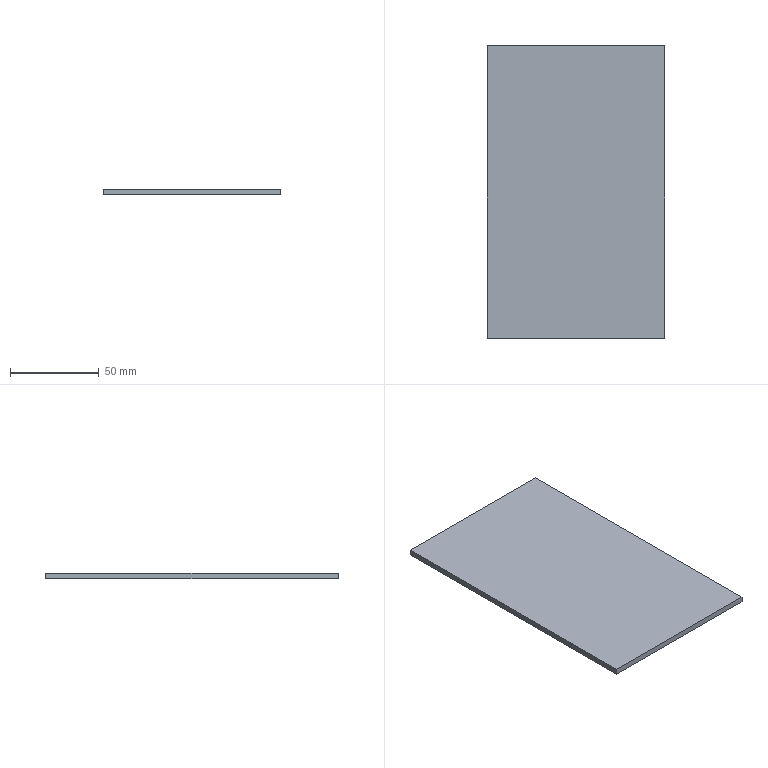Part | STEP file | DMG10600T070_01WTC_X2_8FEA658_5 | 1 solid | 11 faces | box 99.96 x 164.86 x 3.3 mm | volume 52395 mm3 | plane 11
STEP:
#1=CARTESIAN_POINT('',(0.,0.,0.));
#2=DIRECTION('',(0.,0.,1.));
#3=DIRECTION('',(1.,0.,0.));
#4=AXIS2_PLACEMENT_3D('',#1,#2,#3);
#5=CARTESIAN_POINT('',(-49.977,-82.428,-5.7));
#6=VERTEX_POINT('',#5);
#7=CARTESIAN_POINT('',(49.983,-82.428,-5.7));
#8=VERTEX_POINT('',#7);
#9=CARTESIAN_POINT('',(-49.977,-82.428,-5.7));
#10=DIRECTION('',(1.,0.,0.));
#11=VECTOR('',#10,1.);
#12=LINE('',#9,#11);
#13=CARTESIAN_POINT('',(425.814,-2378.632,-5.7));
#14=DIRECTION('',(0.,0.,-1.));
#15=DIRECTION('',(0.,-1.,0.));
#16=AXIS2_PLACEMENT_3D('',#13,#14,#15);
#17=PLANE('',#16);
#18=CARTESIAN_POINT('',(-2296.204,475.791));
#19=DIRECTION('',(0.,-1.));
#20=VECTOR('',#19,1.);
#21=LINE('',#18,#20);
#22=(GEOMETRIC_REPRESENTATION_CONTEXT(2)PARAMETRIC_REPRESENTATION_CONTEXT()REPRESENTATION_CONTEXT('',''));
#23=DEFINITIONAL_REPRESENTATION('',(#21),#22);
#24=PCURVE('',#17,#23);
#25=CARTESIAN_POINT('',(49.983,-82.428,-5.7));
#26=DIRECTION('',(0.,-1.,0.));
#27=DIRECTION('',(1.,0.,0.));
#28=AXIS2_PLACEMENT_3D('',#25,#26,#27);
#29=PLANE('',#28);
#30=CARTESIAN_POINT('',(-99.96,0.));
#31=DIRECTION('',(1.,0.));
#32=VECTOR('',#31,1.);
#33=LINE('',#30,#32);
#34=(GEOMETRIC_REPRESENTATION_CONTEXT(2)PARAMETRIC_REPRESENTATION_CONTEXT()REPRESENTATION_CONTEXT('',''));
#35=DEFINITIONAL_REPRESENTATION('',(#33),#34);
#36=PCURVE('',#29,#35);
#37=SURFACE_CURVE('',#12,(#24,#36),.PCURVE_S1.);
#38=EDGE_CURVE('',#6,#8,#37,.T.);
#39=ORIENTED_EDGE('',*,*,#38,.T.);
#40=CARTESIAN_POINT('',(49.983,82.432,-5.7));
#41=VERTEX_POINT('',#40);
#42=CARTESIAN_POINT('',(49.983,-82.428,-5.7));
#43=DIRECTION('',(0.,1.,0.));
#44=VECTOR('',#43,1.);
#45=LINE('',#42,#44);
#46=CARTESIAN_POINT('',(-2296.204,375.831));
#47=DIRECTION('',(-1.,0.));
#48=VECTOR('',#47,1.);
#49=LINE('',#46,#48);
#50=(GEOMETRIC_REPRESENTATION_CONTEXT(2)PARAMETRIC_REPRESENTATION_CONTEXT()REPRESENTATION_CONTEXT('',''));
#51=DEFINITIONAL_REPRESENTATION('',(#49),#50);
#52=PCURVE('',#17,#51);
#53=CARTESIAN_POINT('',(49.983,82.432,-5.7));
#54=DIRECTION('',(1.,0.,0.));
#55=DIRECTION('',(0.,1.,0.));
#56=AXIS2_PLACEMENT_3D('',#53,#54,#55);
#57=PLANE('',#56);
#58=CARTESIAN_POINT('',(-164.86,0.));
#59=DIRECTION('',(1.,0.));
#60=VECTOR('',#59,1.);
#61=LINE('',#58,#60);
#62=(GEOMETRIC_REPRESENTATION_CONTEXT(2)PARAMETRIC_REPRESENTATION_CONTEXT()REPRESENTATION_CONTEXT('',''));
#63=DEFINITIONAL_REPRESENTATION('',(#61),#62);
#64=PCURVE('',#57,#63);
#65=SURFACE_CURVE('',#45,(#52,#64),.PCURVE_S1.);
#66=EDGE_CURVE('',#8,#41,#65,.T.);
#67=ORIENTED_EDGE('',*,*,#66,.T.);
#68=CARTESIAN_POINT('',(-49.977,82.432,-5.7));
#69=VERTEX_POINT('',#68);
#70=CARTESIAN_POINT('',(49.983,82.432,-5.7));
#71=DIRECTION('',(-1.,0.,0.));
#72=VECTOR('',#71,1.);
#73=LINE('',#70,#72);
#74=CARTESIAN_POINT('',(-2461.064,375.831));
#75=DIRECTION('',(0.,1.));
#76=VECTOR('',#75,1.);
#77=LINE('',#74,#76);
#78=(GEOMETRIC_REPRESENTATION_CONTEXT(2)PARAMETRIC_REPRESENTATION_CONTEXT()REPRESENTATION_CONTEXT('',''));
#79=DEFINITIONAL_REPRESENTATION('',(#77),#78);
#80=PCURVE('',#17,#79);
#81=CARTESIAN_POINT('',(-49.977,82.432,-5.7));
#82=DIRECTION('',(0.,1.,0.));
#83=DIRECTION('',(-1.,0.,0.));
#84=AXIS2_PLACEMENT_3D('',#81,#82,#83);
#85=PLANE('',#84);
#86=CARTESIAN_POINT('',(-99.96,0.));
#87=DIRECTION('',(1.,0.));
#88=VECTOR('',#87,1.);
#89=LINE('',#86,#88);
#90=(GEOMETRIC_REPRESENTATION_CONTEXT(2)PARAMETRIC_REPRESENTATION_CONTEXT()REPRESENTATION_CONTEXT('',''));
#91=DEFINITIONAL_REPRESENTATION('',(#89),#90);
#92=PCURVE('',#85,#91);
#93=SURFACE_CURVE('',#73,(#80,#92),.PCURVE_S1.);
#94=EDGE_CURVE('',#41,#69,#93,.T.);
#95=ORIENTED_EDGE('',*,*,#94,.T.);
#96=CARTESIAN_POINT('',(-49.977,82.432,-5.7));
#97=DIRECTION('',(0.,-1.,0.));
#98=VECTOR('',#97,1.);
#99=LINE('',#96,#98);
#100=CARTESIAN_POINT('',(-2461.064,475.791));
#101=DIRECTION('',(1.,0.));
#102=VECTOR('',#101,1.);
#103=LINE('',#100,#102);
#104=(GEOMETRIC_REPRESENTATION_CONTEXT(2)PARAMETRIC_REPRESENTATION_CONTEXT()REPRESENTATION_CONTEXT('',''));
#105=DEFINITIONAL_REPRESENTATION('',(#103),#104);
#106=PCURVE('',#17,#105);
#107=CARTESIAN_POINT('',(-49.977,-82.428,-5.7));
#108=DIRECTION('',(-1.,0.,0.));
#109=DIRECTION('',(0.,-1.,0.));
#110=AXIS2_PLACEMENT_3D('',#107,#108,#109);
#111=PLANE('',#110);
#112=CARTESIAN_POINT('',(-164.86,0.));
#113=DIRECTION('',(1.,0.));
#114=VECTOR('',#113,1.);
#115=LINE('',#112,#114);
#116=(GEOMETRIC_REPRESENTATION_CONTEXT(2)PARAMETRIC_REPRESENTATION_CONTEXT()REPRESENTATION_CONTEXT('',''));
#117=DEFINITIONAL_REPRESENTATION('',(#115),#116);
#118=PCURVE('',#111,#117);
#119=SURFACE_CURVE('',#99,(#106,#118),.PCURVE_S1.);
#120=EDGE_CURVE('',#69,#6,#119,.T.);
#121=ORIENTED_EDGE('',*,*,#120,.T.);
#122=EDGE_LOOP('',(#39,#67,#95,#121));
#123=FACE_BOUND('',#122,.F.);
#124=CARTESIAN_POINT('',(45.113,-78.905,-5.7));
#125=VERTEX_POINT('',#124);
#126=CARTESIAN_POINT('',(45.113,75.309,-5.7));
#127=VERTEX_POINT('',#126);
#128=CARTESIAN_POINT('',(45.113,-78.905,-5.7));
#129=DIRECTION('',(0.,1.,0.));
#130=VECTOR('',#129,1.);
#131=LINE('',#128,#130);
#132=CARTESIAN_POINT('',(-2299.727,380.701));
#133=DIRECTION('',(-1.,0.));
#134=VECTOR('',#133,1.);
#135=LINE('',#132,#134);
#136=(GEOMETRIC_REPRESENTATION_CONTEXT(2)PARAMETRIC_REPRESENTATION_CONTEXT()REPRESENTATION_CONTEXT('',''));
#137=DEFINITIONAL_REPRESENTATION('',(#135),#136);
#138=PCURVE('',#17,#137);
#139=CARTESIAN_POINT('',(45.113,75.309,-5.7));
#140=DIRECTION('',(1.,0.,0.));
#141=DIRECTION('',(0.,1.,0.));
#142=AXIS2_PLACEMENT_3D('',#139,#140,#141);
#143=PLANE('',#142);
#144=CARTESIAN_POINT('',(-154.214,0.));
#145=DIRECTION('',(1.,0.));
#146=VECTOR('',#145,1.);
#147=LINE('',#144,#146);
#148=(GEOMETRIC_REPRESENTATION_CONTEXT(2)PARAMETRIC_REPRESENTATION_CONTEXT()REPRESENTATION_CONTEXT('',''));
#149=DEFINITIONAL_REPRESENTATION('',(#147),#148);
#150=PCURVE('',#143,#149);
#151=SURFACE_CURVE('',#131,(#138,#150),.PCURVE_S1.);
#152=EDGE_CURVE('',#125,#127,#151,.T.);
#153=ORIENTED_EDGE('',*,*,#152,.F.);
#154=CARTESIAN_POINT('',(-40.807,-78.905,-5.7));
#155=VERTEX_POINT('',#154);
#156=CARTESIAN_POINT('',(-40.807,-78.905,-5.7));
#157=DIRECTION('',(1.,0.,0.));
#158=VECTOR('',#157,1.);
#159=LINE('',#156,#158);
#160=CARTESIAN_POINT('',(-2299.727,466.621));
#161=DIRECTION('',(0.,-1.));
#162=VECTOR('',#161,1.);
#163=LINE('',#160,#162);
#164=(GEOMETRIC_REPRESENTATION_CONTEXT(2)PARAMETRIC_REPRESENTATION_CONTEXT()REPRESENTATION_CONTEXT('',''));
#165=DEFINITIONAL_REPRESENTATION('',(#163),#164);
#166=PCURVE('',#17,#165);
#167=CARTESIAN_POINT('',(45.113,-78.905,-5.7));
#168=DIRECTION('',(0.,-1.,0.));
#169=DIRECTION('',(1.,0.,0.));
#170=AXIS2_PLACEMENT_3D('',#167,#168,#169);
#171=PLANE('',#170);
#172=CARTESIAN_POINT('',(-85.92,0.));
#173=DIRECTION('',(1.,0.));
#174=VECTOR('',#173,1.);
#175=LINE('',#172,#174);
#176=(GEOMETRIC_REPRESENTATION_CONTEXT(2)PARAMETRIC_REPRESENTATION_CONTEXT()REPRESENTATION_CONTEXT('',''));
#177=DEFINITIONAL_REPRESENTATION('',(#175),#176);
#178=PCURVE('',#171,#177);
#179=SURFACE_CURVE('',#159,(#166,#178),.PCURVE_S1.);
#180=EDGE_CURVE('',#155,#125,#179,.T.);
#181=ORIENTED_EDGE('',*,*,#180,.F.);
#182=CARTESIAN_POINT('',(-40.807,75.309,-5.7));
#183=VERTEX_POINT('',#182);
#184=CARTESIAN_POINT('',(-40.807,75.309,-5.7));
#185=DIRECTION('',(0.,-1.,0.));
#186=VECTOR('',#185,1.);
#187=LINE('',#184,#186);
#188=CARTESIAN_POINT('',(-2453.941,466.621));
#189=DIRECTION('',(1.,0.));
#190=VECTOR('',#189,1.);
#191=LINE('',#188,#190);
#192=(GEOMETRIC_REPRESENTATION_CONTEXT(2)PARAMETRIC_REPRESENTATION_CONTEXT()REPRESENTATION_CONTEXT('',''));
#193=DEFINITIONAL_REPRESENTATION('',(#191),#192);
#194=PCURVE('',#17,#193);
#195=CARTESIAN_POINT('',(-40.807,-78.905,-5.7));
#196=DIRECTION('',(-1.,0.,0.));
#197=DIRECTION('',(0.,-1.,0.));
#198=AXIS2_PLACEMENT_3D('',#195,#196,#197);
#199=PLANE('',#198);
#200=CARTESIAN_POINT('',(-154.214,0.));
#201=DIRECTION('',(1.,0.));
#202=VECTOR('',#201,1.);
#203=LINE('',#200,#202);
#204=(GEOMETRIC_REPRESENTATION_CONTEXT(2)PARAMETRIC_REPRESENTATION_CONTEXT()REPRESENTATION_CONTEXT('',''));
#205=DEFINITIONAL_REPRESENTATION('',(#203),#204);
#206=PCURVE('',#199,#205);
#207=SURFACE_CURVE('',#187,(#194,#206),.PCURVE_S1.);
#208=EDGE_CURVE('',#183,#155,#207,.T.);
#209=ORIENTED_EDGE('',*,*,#208,.F.);
#210=CARTESIAN_POINT('',(45.113,75.309,-5.7));
#211=DIRECTION('',(-1.,0.,0.));
#212=VECTOR('',#211,1.);
#213=LINE('',#210,#212);
#214=CARTESIAN_POINT('',(-2453.941,380.701));
#215=DIRECTION('',(0.,1.));
#216=VECTOR('',#215,1.);
#217=LINE('',#214,#216);
#218=(GEOMETRIC_REPRESENTATION_CONTEXT(2)PARAMETRIC_REPRESENTATION_CONTEXT()REPRESENTATION_CONTEXT('',''));
#219=DEFINITIONAL_REPRESENTATION('',(#217),#218);
#220=PCURVE('',#17,#219);
#221=CARTESIAN_POINT('',(-40.807,75.309,-5.7));
#222=DIRECTION('',(0.,1.,0.));
#223=DIRECTION('',(-1.,0.,0.));
#224=AXIS2_PLACEMENT_3D('',#221,#222,#223);
#225=PLANE('',#224);
#226=CARTESIAN_POINT('',(-85.92,0.));
#227=DIRECTION('',(1.,0.));
#228=VECTOR('',#227,1.);
#229=LINE('',#226,#228);
#230=(GEOMETRIC_REPRESENTATION_CONTEXT(2)PARAMETRIC_REPRESENTATION_CONTEXT()REPRESENTATION_CONTEXT('',''));
#231=DEFINITIONAL_REPRESENTATION('',(#229),#230);
#232=PCURVE('',#225,#231);
#233=SURFACE_CURVE('',#213,(#220,#232),.PCURVE_S1.);
#234=EDGE_CURVE('',#127,#183,#233,.T.);
#235=ORIENTED_EDGE('',*,*,#234,.F.);
#236=EDGE_LOOP('',(#153,#181,#209,#235));
#237=FACE_BOUND('',#236,.F.);
#238=ADVANCED_FACE('',(#123,#237),#17,.T.);
#239=CARTESIAN_POINT('',(49.983,-82.428,-2.4));
#240=VERTEX_POINT('',#239);
#241=CARTESIAN_POINT('',(49.983,-82.428,-2.4));
#242=DIRECTION('',(0.,0.,-1.));
#243=VECTOR('',#242,1.);
#244=LINE('',#241,#243);
#245=CARTESIAN_POINT('',(0.,3.3));
#246=DIRECTION('',(0.,-1.));
#247=VECTOR('',#246,1.);
#248=LINE('',#245,#247);
#249=(GEOMETRIC_REPRESENTATION_CONTEXT(2)PARAMETRIC_REPRESENTATION_CONTEXT()REPRESENTATION_CONTEXT('',''));
#250=DEFINITIONAL_REPRESENTATION('',(#248),#249);
#251=PCURVE('',#29,#250);
#252=CARTESIAN_POINT('',(-164.86,3.3));
#253=DIRECTION('',(0.,-1.));
#254=VECTOR('',#253,1.);
#255=LINE('',#252,#254);
#256=(GEOMETRIC_REPRESENTATION_CONTEXT(2)PARAMETRIC_REPRESENTATION_CONTEXT()REPRESENTATION_CONTEXT('',''));
#257=DEFINITIONAL_REPRESENTATION('',(#255),#256);
#258=PCURVE('',#57,#257);
#259=SURFACE_CURVE('',#244,(#251,#258),.PCURVE_S1.);
#260=EDGE_CURVE('',#240,#8,#259,.T.);
#261=ORIENTED_EDGE('',*,*,#260,.T.);
#262=ORIENTED_EDGE('',*,*,#38,.F.);
#263=CARTESIAN_POINT('',(-49.977,-82.428,-2.4));
#264=VERTEX_POINT('',#263);
#265=CARTESIAN_POINT('',(-49.977,-82.428,-2.4));
#266=DIRECTION('',(0.,0.,-1.));
#267=VECTOR('',#266,1.);
#268=LINE('',#265,#267);
#269=CARTESIAN_POINT('',(-99.96,3.3));
#270=DIRECTION('',(0.,-1.));
#271=VECTOR('',#270,1.);
#272=LINE('',#269,#271);
#273=(GEOMETRIC_REPRESENTATION_CONTEXT(2)PARAMETRIC_REPRESENTATION_CONTEXT()REPRESENTATION_CONTEXT('',''));
#274=DEFINITIONAL_REPRESENTATION('',(#272),#273);
#275=PCURVE('',#29,#274);
#276=CARTESIAN_POINT('',(0.,3.3));
#277=DIRECTION('',(0.,-1.));
#278=VECTOR('',#277,1.);
#279=LINE('',#276,#278);
#280=(GEOMETRIC_REPRESENTATION_CONTEXT(2)PARAMETRIC_REPRESENTATION_CONTEXT()REPRESENTATION_CONTEXT('',''));
#281=DEFINITIONAL_REPRESENTATION('',(#279),#280);
#282=PCURVE('',#111,#281);
#283=SURFACE_CURVE('',#268,(#275,#282),.PCURVE_S1.);
#284=EDGE_CURVE('',#264,#6,#283,.T.);
#285=ORIENTED_EDGE('',*,*,#284,.F.);
#286=CARTESIAN_POINT('',(-49.977,-82.428,-2.4));
#287=DIRECTION('',(1.,0.,0.));
#288=VECTOR('',#287,1.);
#289=LINE('',#286,#288);
#290=CARTESIAN_POINT('',(-99.96,3.3));
#291=DIRECTION('',(1.,0.));
#292=VECTOR('',#291,1.);
#293=LINE('',#290,#292);
#294=(GEOMETRIC_REPRESENTATION_CONTEXT(2)PARAMETRIC_REPRESENTATION_CONTEXT()REPRESENTATION_CONTEXT('',''));
#295=DEFINITIONAL_REPRESENTATION('',(#293),#294);
#296=PCURVE('',#29,#295);
#297=CARTESIAN_POINT('',(425.814,-2378.632,-2.4));
#298=DIRECTION('',(0.,0.,-1.));
#299=DIRECTION('',(0.,-1.,0.));
#300=AXIS2_PLACEMENT_3D('',#297,#298,#299);
#301=PLANE('',#300);
#302=CARTESIAN_POINT('',(-2296.204,475.791));
#303=DIRECTION('',(0.,-1.));
#304=VECTOR('',#303,1.);
#305=LINE('',#302,#304);
#306=(GEOMETRIC_REPRESENTATION_CONTEXT(2)PARAMETRIC_REPRESENTATION_CONTEXT()REPRESENTATION_CONTEXT('',''));
#307=DEFINITIONAL_REPRESENTATION('',(#305),#306);
#308=PCURVE('',#301,#307);
#309=SURFACE_CURVE('',#289,(#296,#308),.PCURVE_S1.);
#310=EDGE_CURVE('',#264,#240,#309,.T.);
#311=ORIENTED_EDGE('',*,*,#310,.T.);
#312=EDGE_LOOP('',(#261,#262,#285,#311));
#313=FACE_BOUND('',#312,.F.);
#314=ADVANCED_FACE('',(#313),#29,.T.);
#315=CARTESIAN_POINT('',(49.983,82.432,-2.4));
#316=VERTEX_POINT('',#315);
#317=CARTESIAN_POINT('',(49.983,82.432,-2.4));
#318=DIRECTION('',(0.,0.,-1.));
#319=VECTOR('',#318,1.);
#320=LINE('',#317,#319);
#321=CARTESIAN_POINT('',(0.,3.3));
#322=DIRECTION('',(0.,-1.));
#323=VECTOR('',#322,1.);
#324=LINE('',#321,#323);
#325=(GEOMETRIC_REPRESENTATION_CONTEXT(2)PARAMETRIC_REPRESENTATION_CONTEXT()REPRESENTATION_CONTEXT('',''));
#326=DEFINITIONAL_REPRESENTATION('',(#324),#325);
#327=PCURVE('',#57,#326);
#328=CARTESIAN_POINT('',(-99.96,3.3));
#329=DIRECTION('',(0.,-1.));
#330=VECTOR('',#329,1.);
#331=LINE('',#328,#330);
#332=(GEOMETRIC_REPRESENTATION_CONTEXT(2)PARAMETRIC_REPRESENTATION_CONTEXT()REPRESENTATION_CONTEXT('',''));
#333=DEFINITIONAL_REPRESENTATION('',(#331),#332);
#334=PCURVE('',#85,#333);
#335=SURFACE_CURVE('',#320,(#327,#334),.PCURVE_S1.);
#336=EDGE_CURVE('',#316,#41,#335,.T.);
#337=ORIENTED_EDGE('',*,*,#336,.T.);
#338=ORIENTED_EDGE('',*,*,#66,.F.);
#339=ORIENTED_EDGE('',*,*,#260,.F.);
#340=CARTESIAN_POINT('',(49.983,-82.428,-2.4));
#341=DIRECTION('',(0.,1.,0.));
#342=VECTOR('',#341,1.);
#343=LINE('',#340,#342);
#344=CARTESIAN_POINT('',(-164.86,3.3));
#345=DIRECTION('',(1.,0.));
#346=VECTOR('',#345,1.);
#347=LINE('',#344,#346);
#348=(GEOMETRIC_REPRESENTATION_CONTEXT(2)PARAMETRIC_REPRESENTATION_CONTEXT()REPRESENTATION_CONTEXT('',''));
#349=DEFINITIONAL_REPRESENTATION('',(#347),#348);
#350=PCURVE('',#57,#349);
#351=CARTESIAN_POINT('',(-2296.204,375.831));
#352=DIRECTION('',(-1.,0.));
#353=VECTOR('',#352,1.);
#354=LINE('',#351,#353);
#355=(GEOMETRIC_REPRESENTATION_CONTEXT(2)PARAMETRIC_REPRESENTATION_CONTEXT()REPRESENTATION_CONTEXT('',''));
#356=DEFINITIONAL_REPRESENTATION('',(#354),#355);
#357=PCURVE('',#301,#356);
#358=SURFACE_CURVE('',#343,(#350,#357),.PCURVE_S1.);
#359=EDGE_CURVE('',#240,#316,#358,.T.);
#360=ORIENTED_EDGE('',*,*,#359,.T.);
#361=EDGE_LOOP('',(#337,#338,#339,#360));
#362=FACE_BOUND('',#361,.F.);
#363=ADVANCED_FACE('',(#362),#57,.T.);
#364=CARTESIAN_POINT('',(-49.977,82.432,-2.4));
#365=VERTEX_POINT('',#364);
#366=CARTESIAN_POINT('',(-49.977,82.432,-2.4));
#367=DIRECTION('',(0.,0.,-1.));
#368=VECTOR('',#367,1.);
#369=LINE('',#366,#368);
#370=CARTESIAN_POINT('',(0.,3.3));
#371=DIRECTION('',(0.,-1.));
#372=VECTOR('',#371,1.);
#373=LINE('',#370,#372);
#374=(GEOMETRIC_REPRESENTATION_CONTEXT(2)PARAMETRIC_REPRESENTATION_CONTEXT()REPRESENTATION_CONTEXT('',''));
#375=DEFINITIONAL_REPRESENTATION('',(#373),#374);
#376=PCURVE('',#85,#375);
#377=CARTESIAN_POINT('',(-164.86,3.3));
#378=DIRECTION('',(0.,-1.));
#379=VECTOR('',#378,1.);
#380=LINE('',#377,#379);
#381=(GEOMETRIC_REPRESENTATION_CONTEXT(2)PARAMETRIC_REPRESENTATION_CONTEXT()REPRESENTATION_CONTEXT('',''));
#382=DEFINITIONAL_REPRESENTATION('',(#380),#381);
#383=PCURVE('',#111,#382);
#384=SURFACE_CURVE('',#369,(#376,#383),.PCURVE_S1.);
#385=EDGE_CURVE('',#365,#69,#384,.T.);
#386=ORIENTED_EDGE('',*,*,#385,.T.);
#387=ORIENTED_EDGE('',*,*,#94,.F.);
#388=ORIENTED_EDGE('',*,*,#336,.F.);
#389=CARTESIAN_POINT('',(49.983,82.432,-2.4));
#390=DIRECTION('',(-1.,0.,0.));
#391=VECTOR('',#390,1.);
#392=LINE('',#389,#391);
#393=CARTESIAN_POINT('',(-99.96,3.3));
#394=DIRECTION('',(1.,0.));
#395=VECTOR('',#394,1.);
#396=LINE('',#393,#395);
#397=(GEOMETRIC_REPRESENTATION_CONTEXT(2)PARAMETRIC_REPRESENTATION_CONTEXT()REPRESENTATION_CONTEXT('',''));
#398=DEFINITIONAL_REPRESENTATION('',(#396),#397);
#399=PCURVE('',#85,#398);
#400=CARTESIAN_POINT('',(-2461.064,375.831));
#401=DIRECTION('',(0.,1.));
#402=VECTOR('',#401,1.);
#403=LINE('',#400,#402);
#404=(GEOMETRIC_REPRESENTATION_CONTEXT(2)PARAMETRIC_REPRESENTATION_CONTEXT()REPRESENTATION_CONTEXT('',''));
#405=DEFINITIONAL_REPRESENTATION('',(#403),#404);
#406=PCURVE('',#301,#405);
#407=SURFACE_CURVE('',#392,(#399,#406),.PCURVE_S1.);
#408=EDGE_CURVE('',#316,#365,#407,.T.);
#409=ORIENTED_EDGE('',*,*,#408,.T.);
#410=EDGE_LOOP('',(#386,#387,#388,#409));
#411=FACE_BOUND('',#410,.F.);
#412=ADVANCED_FACE('',(#411),#85,.T.);
#413=ORIENTED_EDGE('',*,*,#284,.T.);
#414=ORIENTED_EDGE('',*,*,#120,.F.);
#415=ORIENTED_EDGE('',*,*,#385,.F.);
#416=CARTESIAN_POINT('',(-49.977,82.432,-2.4));
#417=DIRECTION('',(0.,-1.,0.));
#418=VECTOR('',#417,1.);
#419=LINE('',#416,#418);
#420=CARTESIAN_POINT('',(-164.86,3.3));
#421=DIRECTION('',(1.,0.));
#422=VECTOR('',#421,1.);
#423=LINE('',#420,#422);
#424=(GEOMETRIC_REPRESENTATION_CONTEXT(2)PARAMETRIC_REPRESENTATION_CONTEXT()REPRESENTATION_CONTEXT('',''));
#425=DEFINITIONAL_REPRESENTATION('',(#423),#424);
#426=PCURVE('',#111,#425);
#427=CARTESIAN_POINT('',(-2461.064,475.791));
#428=DIRECTION('',(1.,0.));
#429=VECTOR('',#428,1.);
#430=LINE('',#427,#429);
#431=(GEOMETRIC_REPRESENTATION_CONTEXT(2)PARAMETRIC_REPRESENTATION_CONTEXT()REPRESENTATION_CONTEXT('',''));
#432=DEFINITIONAL_REPRESENTATION('',(#430),#431);
#433=PCURVE('',#301,#432);
#434=SURFACE_CURVE('',#419,(#426,#433),.PCURVE_S1.);
#435=EDGE_CURVE('',#365,#264,#434,.T.);
#436=ORIENTED_EDGE('',*,*,#435,.T.);
#437=EDGE_LOOP('',(#413,#414,#415,#436));
#438=FACE_BOUND('',#437,.F.);
#439=ADVANCED_FACE('',(#438),#111,.T.);
#440=ORIENTED_EDGE('',*,*,#408,.F.);
#441=ORIENTED_EDGE('',*,*,#359,.F.);
#442=ORIENTED_EDGE('',*,*,#310,.F.);
#443=ORIENTED_EDGE('',*,*,#435,.F.);
#444=EDGE_LOOP('',(#440,#441,#442,#443));
#445=FACE_BOUND('',#444,.F.);
#446=ADVANCED_FACE('',(#445),#301,.F.);
#447=CARTESIAN_POINT('',(45.113,-78.905,-5.55));
#448=VERTEX_POINT('',#447);
#449=CARTESIAN_POINT('',(45.113,-78.905,-5.55));
#450=DIRECTION('',(0.,0.,-1.));
#451=VECTOR('',#450,1.);
#452=LINE('',#449,#451);
#453=CARTESIAN_POINT('',(-154.214,0.15));
#454=DIRECTION('',(0.,-1.));
#455=VECTOR('',#454,1.);
#456=LINE('',#453,#455);
#457=(GEOMETRIC_REPRESENTATION_CONTEXT(2)PARAMETRIC_REPRESENTATION_CONTEXT()REPRESENTATION_CONTEXT('',''));
#458=DEFINITIONAL_REPRESENTATION('',(#456),#457);
#459=PCURVE('',#143,#458);
#460=CARTESIAN_POINT('',(0.,0.15));
#461=DIRECTION('',(0.,-1.));
#462=VECTOR('',#461,1.);
#463=LINE('',#460,#462);
#464=(GEOMETRIC_REPRESENTATION_CONTEXT(2)PARAMETRIC_REPRESENTATION_CONTEXT()REPRESENTATION_CONTEXT('',''));
#465=DEFINITIONAL_REPRESENTATION('',(#463),#464);
#466=PCURVE('',#171,#465);
#467=SURFACE_CURVE('',#452,(#459,#466),.PCURVE_S1.);
#468=EDGE_CURVE('',#448,#125,#467,.T.);
#469=ORIENTED_EDGE('',*,*,#468,.T.);
#470=ORIENTED_EDGE('',*,*,#152,.T.);
#471=CARTESIAN_POINT('',(45.113,75.309,-5.55));
#472=VERTEX_POINT('',#471);
#473=CARTESIAN_POINT('',(45.113,75.309,-5.55));
#474=DIRECTION('',(0.,0.,-1.));
#475=VECTOR('',#474,1.);
#476=LINE('',#473,#475);
#477=CARTESIAN_POINT('',(0.,0.15));
#478=DIRECTION('',(0.,-1.));
#479=VECTOR('',#478,1.);
#480=LINE('',#477,#479);
#481=(GEOMETRIC_REPRESENTATION_CONTEXT(2)PARAMETRIC_REPRESENTATION_CONTEXT()REPRESENTATION_CONTEXT('',''));
#482=DEFINITIONAL_REPRESENTATION('',(#480),#481);
#483=PCURVE('',#143,#482);
#484=CARTESIAN_POINT('',(-85.92,0.15));
#485=DIRECTION('',(0.,-1.));
#486=VECTOR('',#485,1.);
#487=LINE('',#484,#486);
#488=(GEOMETRIC_REPRESENTATION_CONTEXT(2)PARAMETRIC_REPRESENTATION_CONTEXT()REPRESENTATION_CONTEXT('',''));
#489=DEFINITIONAL_REPRESENTATION('',(#487),#488);
#490=PCURVE('',#225,#489);
#491=SURFACE_CURVE('',#476,(#483,#490),.PCURVE_S1.);
#492=EDGE_CURVE('',#472,#127,#491,.T.);
#493=ORIENTED_EDGE('',*,*,#492,.F.);
#494=CARTESIAN_POINT('',(45.113,-78.905,-5.55));
#495=DIRECTION('',(0.,1.,0.));
#496=VECTOR('',#495,1.);
#497=LINE('',#494,#496);
#498=CARTESIAN_POINT('',(-154.214,0.15));
#499=DIRECTION('',(1.,0.));
#500=VECTOR('',#499,1.);
#501=LINE('',#498,#500);
#502=(GEOMETRIC_REPRESENTATION_CONTEXT(2)PARAMETRIC_REPRESENTATION_CONTEXT()REPRESENTATION_CONTEXT('',''));
#503=DEFINITIONAL_REPRESENTATION('',(#501),#502);
#504=PCURVE('',#143,#503);
#505=CARTESIAN_POINT('',(-49.977,-82.428,-5.55));
#506=DIRECTION('',(0.,0.,-1.));
#507=DIRECTION('',(0.,-1.,0.));
#508=AXIS2_PLACEMENT_3D('',#505,#506,#507);
#509=PLANE('',#508);
#510=CARTESIAN_POINT('',(-3.523,-95.09));
#511=DIRECTION('',(-1.,0.));
#512=VECTOR('',#511,1.);
#513=LINE('',#510,#512);
#514=(GEOMETRIC_REPRESENTATION_CONTEXT(2)PARAMETRIC_REPRESENTATION_CONTEXT()REPRESENTATION_CONTEXT('',''));
#515=DEFINITIONAL_REPRESENTATION('',(#513),#514);
#516=PCURVE('',#509,#515);
#517=SURFACE_CURVE('',#497,(#504,#516),.PCURVE_S1.);
#518=EDGE_CURVE('',#448,#472,#517,.T.);
#519=ORIENTED_EDGE('',*,*,#518,.F.);
#520=EDGE_LOOP('',(#469,#470,#493,#519));
#521=FACE_BOUND('',#520,.F.);
#522=ADVANCED_FACE('',(#521),#143,.F.);
#523=CARTESIAN_POINT('',(-40.807,-78.905,-5.55));
#524=VERTEX_POINT('',#523);
#525=CARTESIAN_POINT('',(-40.807,-78.905,-5.55));
#526=DIRECTION('',(0.,0.,-1.));
#527=VECTOR('',#526,1.);
#528=LINE('',#525,#527);
#529=CARTESIAN_POINT('',(-85.92,0.15));
#530=DIRECTION('',(0.,-1.));
#531=VECTOR('',#530,1.);
#532=LINE('',#529,#531);
#533=(GEOMETRIC_REPRESENTATION_CONTEXT(2)PARAMETRIC_REPRESENTATION_CONTEXT()REPRESENTATION_CONTEXT('',''));
#534=DEFINITIONAL_REPRESENTATION('',(#532),#533);
#535=PCURVE('',#171,#534);
#536=CARTESIAN_POINT('',(0.,0.15));
#537=DIRECTION('',(0.,-1.));
#538=VECTOR('',#537,1.);
#539=LINE('',#536,#538);
#540=(GEOMETRIC_REPRESENTATION_CONTEXT(2)PARAMETRIC_REPRESENTATION_CONTEXT()REPRESENTATION_CONTEXT('',''));
#541=DEFINITIONAL_REPRESENTATION('',(#539),#540);
#542=PCURVE('',#199,#541);
#543=SURFACE_CURVE('',#528,(#535,#542),.PCURVE_S1.);
#544=EDGE_CURVE('',#524,#155,#543,.T.);
#545=ORIENTED_EDGE('',*,*,#544,.T.);
#546=ORIENTED_EDGE('',*,*,#180,.T.);
#547=ORIENTED_EDGE('',*,*,#468,.F.);
#548=CARTESIAN_POINT('',(-40.807,-78.905,-5.55));
#549=DIRECTION('',(1.,0.,0.));
#550=VECTOR('',#549,1.);
#551=LINE('',#548,#550);
#552=CARTESIAN_POINT('',(-85.92,0.15));
#553=DIRECTION('',(1.,0.));
#554=VECTOR('',#553,1.);
#555=LINE('',#552,#554);
#556=(GEOMETRIC_REPRESENTATION_CONTEXT(2)PARAMETRIC_REPRESENTATION_CONTEXT()REPRESENTATION_CONTEXT('',''));
#557=DEFINITIONAL_REPRESENTATION('',(#555),#556);
#558=PCURVE('',#171,#557);
#559=CARTESIAN_POINT('',(-3.523,-9.17));
#560=DIRECTION('',(0.,-1.));
#561=VECTOR('',#560,1.);
#562=LINE('',#559,#561);
#563=(GEOMETRIC_REPRESENTATION_CONTEXT(2)PARAMETRIC_REPRESENTATION_CONTEXT()REPRESENTATION_CONTEXT('',''));
#564=DEFINITIONAL_REPRESENTATION('',(#562),#563);
#565=PCURVE('',#509,#564);
#566=SURFACE_CURVE('',#551,(#558,#565),.PCURVE_S1.);
#567=EDGE_CURVE('',#524,#448,#566,.T.);
#568=ORIENTED_EDGE('',*,*,#567,.F.);
#569=EDGE_LOOP('',(#545,#546,#547,#568));
#570=FACE_BOUND('',#569,.F.);
#571=ADVANCED_FACE('',(#570),#171,.F.);
#572=CARTESIAN_POINT('',(-40.807,75.309,-5.55));
#573=VERTEX_POINT('',#572);
#574=CARTESIAN_POINT('',(-40.807,75.309,-5.55));
#575=DIRECTION('',(0.,0.,-1.));
#576=VECTOR('',#575,1.);
#577=LINE('',#574,#576);
#578=CARTESIAN_POINT('',(-154.214,0.15));
#579=DIRECTION('',(0.,-1.));
#580=VECTOR('',#579,1.);
#581=LINE('',#578,#580);
#582=(GEOMETRIC_REPRESENTATION_CONTEXT(2)PARAMETRIC_REPRESENTATION_CONTEXT()REPRESENTATION_CONTEXT('',''));
#583=DEFINITIONAL_REPRESENTATION('',(#581),#582);
#584=PCURVE('',#199,#583);
#585=CARTESIAN_POINT('',(0.,0.15));
#586=DIRECTION('',(0.,-1.));
#587=VECTOR('',#586,1.);
#588=LINE('',#585,#587);
#589=(GEOMETRIC_REPRESENTATION_CONTEXT(2)PARAMETRIC_REPRESENTATION_CONTEXT()REPRESENTATION_CONTEXT('',''));
#590=DEFINITIONAL_REPRESENTATION('',(#588),#589);
#591=PCURVE('',#225,#590);
#592=SURFACE_CURVE('',#577,(#584,#591),.PCURVE_S1.);
#593=EDGE_CURVE('',#573,#183,#592,.T.);
#594=ORIENTED_EDGE('',*,*,#593,.T.);
#595=ORIENTED_EDGE('',*,*,#208,.T.);
#596=ORIENTED_EDGE('',*,*,#544,.F.);
#597=CARTESIAN_POINT('',(-40.807,75.309,-5.55));
#598=DIRECTION('',(0.,-1.,0.));
#599=VECTOR('',#598,1.);
#600=LINE('',#597,#599);
#601=CARTESIAN_POINT('',(-154.214,0.15));
#602=DIRECTION('',(1.,0.));
#603=VECTOR('',#602,1.);
#604=LINE('',#601,#603);
#605=(GEOMETRIC_REPRESENTATION_CONTEXT(2)PARAMETRIC_REPRESENTATION_CONTEXT()REPRESENTATION_CONTEXT('',''));
#606=DEFINITIONAL_REPRESENTATION('',(#604),#605);
#607=PCURVE('',#199,#606);
#608=CARTESIAN_POINT('',(-157.737,-9.17));
#609=DIRECTION('',(1.,0.));
#610=VECTOR('',#609,1.);
#611=LINE('',#608,#610);
#612=(GEOMETRIC_REPRESENTATION_CONTEXT(2)PARAMETRIC_REPRESENTATION_CONTEXT()REPRESENTATION_CONTEXT('',''));
#613=DEFINITIONAL_REPRESENTATION('',(#611),#612);
#614=PCURVE('',#509,#613);
#615=SURFACE_CURVE('',#600,(#607,#614),.PCURVE_S1.);
#616=EDGE_CURVE('',#573,#524,#615,.T.);
#617=ORIENTED_EDGE('',*,*,#616,.F.);
#618=EDGE_LOOP('',(#594,#595,#596,#617));
#619=FACE_BOUND('',#618,.F.);
#620=ADVANCED_FACE('',(#619),#199,.F.);
#621=ORIENTED_EDGE('',*,*,#492,.T.);
#622=ORIENTED_EDGE('',*,*,#234,.T.);
#623=ORIENTED_EDGE('',*,*,#593,.F.);
#624=CARTESIAN_POINT('',(45.113,75.309,-5.55));
#625=DIRECTION('',(-1.,0.,0.));
#626=VECTOR('',#625,1.);
#627=LINE('',#624,#626);
#628=CARTESIAN_POINT('',(-85.92,0.15));
#629=DIRECTION('',(1.,0.));
#630=VECTOR('',#629,1.);
#631=LINE('',#628,#630);
#632=(GEOMETRIC_REPRESENTATION_CONTEXT(2)PARAMETRIC_REPRESENTATION_CONTEXT()REPRESENTATION_CONTEXT('',''));
#633=DEFINITIONAL_REPRESENTATION('',(#631),#632);
#634=PCURVE('',#225,#633);
#635=CARTESIAN_POINT('',(-157.737,-95.09));
#636=DIRECTION('',(0.,1.));
#637=VECTOR('',#636,1.);
#638=LINE('',#635,#637);
#639=(GEOMETRIC_REPRESENTATION_CONTEXT(2)PARAMETRIC_REPRESENTATION_CONTEXT()REPRESENTATION_CONTEXT('',''));
#640=DEFINITIONAL_REPRESENTATION('',(#638),#639);
#641=PCURVE('',#509,#640);
#642=SURFACE_CURVE('',#627,(#634,#641),.PCURVE_S1.);
#643=EDGE_CURVE('',#472,#573,#642,.T.);
#644=ORIENTED_EDGE('',*,*,#643,.F.);
#645=EDGE_LOOP('',(#621,#622,#623,#644));
#646=FACE_BOUND('',#645,.F.);
#647=ADVANCED_FACE('',(#646),#225,.F.);
#648=ORIENTED_EDGE('',*,*,#616,.T.);
#649=ORIENTED_EDGE('',*,*,#567,.T.);
#650=ORIENTED_EDGE('',*,*,#518,.T.);
#651=ORIENTED_EDGE('',*,*,#643,.T.);
#652=EDGE_LOOP('',(#648,#649,#650,#651));
#653=FACE_BOUND('',#652,.F.);
#654=ADVANCED_FACE('',(#653),#509,.T.);
#655=CLOSED_SHELL('',(#238,#314,#363,#412,#439,#446,#522,#571,#620,#647,#654));
#656=MANIFOLD_SOLID_BREP('',#655);
#657=(LENGTH_UNIT()NAMED_UNIT(*)SI_UNIT(.MILLI.,.METRE.));
#658=UNCERTAINTY_MEASURE_WITH_UNIT(LENGTH_MEASURE(0.0000001),#657,'','');
#659=(NAMED_UNIT(*)PLANE_ANGLE_UNIT()SI_UNIT($,.RADIAN.));
#660=(NAMED_UNIT(*)SI_UNIT($,.STERADIAN.)SOLID_ANGLE_UNIT());
#661=(GEOMETRIC_REPRESENTATION_CONTEXT(3)GLOBAL_UNCERTAINTY_ASSIGNED_CONTEXT((#658))GLOBAL_UNIT_ASSIGNED_CONTEXT((#657,#659,#660))REPRESENTATION_CONTEXT('',''));
#662=ADVANCED_BREP_SHAPE_REPRESENTATION('',(#4,#656),#661);